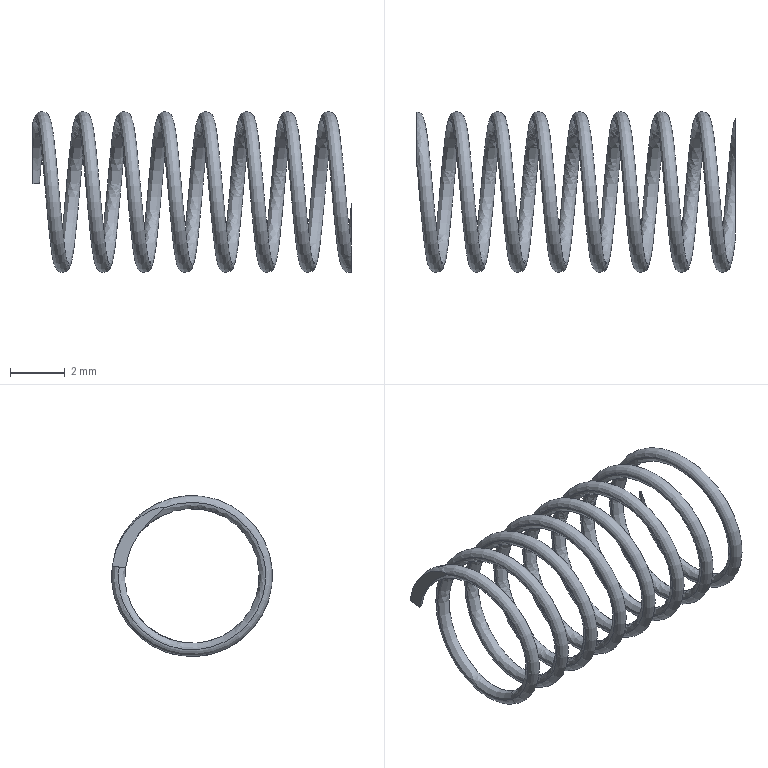Part | SolidWorks | features BaseBody 1 | 1 solid | 5 faces | box 11.683 x 5.9 x 5.9 mm | volume 27.883 mm3 | plane 3 | spline 2